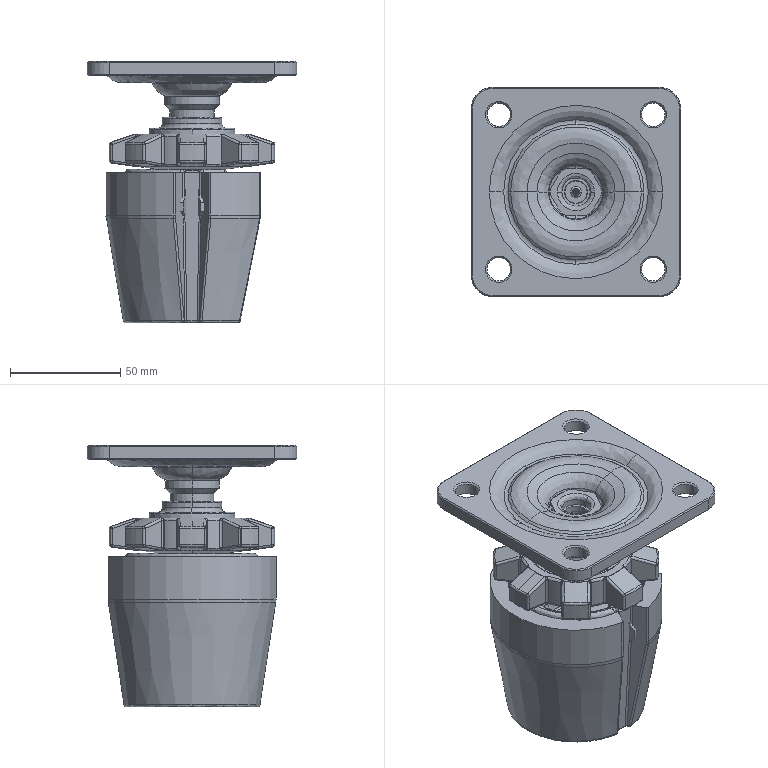Part | SolidWorks | features BaseBody 1 | 1 solid | 1011 faces | box 95 x 95 x 118.5 mm | volume 311521 mm3 | spline 378 | plane 230 | cylinder 226 | cone 152 | torus 25 | commonest cylinder face diameters 2 x92 4 x23 1 x18 10 x11 10.6 x10 20 x10